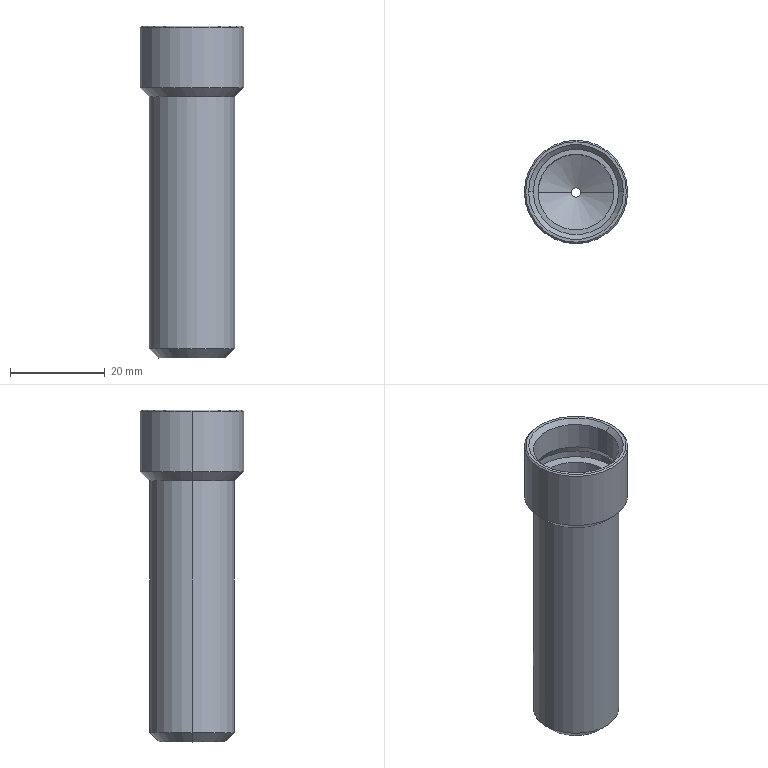Part | SolidWorks | features BaseBody 1 | 1 solid | 27 faces | box 21.8 x 21.8 x 70 mm | volume 5495 mm3 | cylinder 12 | cone 12 | plane 3 | commonest cylinder face diameters 18 x4 2 x2 16 x2 20 x2 21.8 x2
STEP:
#1=CARTESIAN_POINT('',(471.537,37.715,-74.634));
#2=VERTEX_POINT('',#1);
#3=CARTESIAN_POINT('',(489.537,37.715,-74.634));
#4=VERTEX_POINT('',#3);
#5=CARTESIAN_POINT('',(480.537,37.715,-74.634));
#6=DIRECTION('',(0.000000013,0.,-1.));
#7=DIRECTION('',(0.,1.,0.));
#8=AXIS2_PLACEMENT_3D('',#5,#6,#7);
#9=CIRCLE('',#8,9.);
#10=EDGE_CURVE('',#2,#4,#9,.T.);
#11=ORIENTED_EDGE('',*,*,#10,.F.);
#12=CARTESIAN_POINT('',(471.537,37.715,-21.534));
#13=VERTEX_POINT('',#12);
#14=CARTESIAN_POINT('',(471.537,37.715,-74.634));
#15=DIRECTION('',(-0.000000013,0.,1.));
#16=VECTOR('',#15,1000.);
#17=LINE('',#14,#16);
#18=EDGE_CURVE('',#2,#13,#17,.T.);
#19=ORIENTED_EDGE('',*,*,#18,.T.);
#20=CARTESIAN_POINT('',(489.537,37.715,-21.534));
#21=VERTEX_POINT('',#20);
#22=CARTESIAN_POINT('',(480.537,37.715,-21.534));
#23=DIRECTION('',(-0.000000013,0.,1.));
#24=DIRECTION('',(0.,1.,0.));
#25=AXIS2_PLACEMENT_3D('',#22,#23,#24);
#26=CIRCLE('',#25,9.);
#27=EDGE_CURVE('',#21,#13,#26,.T.);
#28=ORIENTED_EDGE('',*,*,#27,.F.);
#29=CARTESIAN_POINT('',(489.537,37.715,-74.634));
#30=DIRECTION('',(-0.000000013,0.,1.));
#31=VECTOR('',#30,1000.);
#32=LINE('',#29,#31);
#33=EDGE_CURVE('',#4,#21,#32,.T.);
#34=ORIENTED_EDGE('',*,*,#33,.F.);
#35=EDGE_LOOP('',(#11,#19,#28,#34));
#36=FACE_OUTER_BOUND('',#35,.T.);
#37=CARTESIAN_POINT('',(480.537,37.715,-74.634));
#38=DIRECTION('',(-0.000000013,0.,1.));
#39=DIRECTION('',(1.,0.,0.000000013));
#40=AXIS2_PLACEMENT_3D('',#37,#38,#39);
#41=CYLINDRICAL_SURFACE('',#40,9.);
#42=ADVANCED_FACE('',(#36),#41,.T.);
#43=CARTESIAN_POINT('',(473.537,37.715,-76.634));
#44=VERTEX_POINT('',#43);
#45=CARTESIAN_POINT('',(487.537,37.715,-76.634));
#46=VERTEX_POINT('',#45);
#47=CARTESIAN_POINT('',(480.537,37.715,-76.634));
#48=DIRECTION('',(0.000000013,0.,-1.));
#49=DIRECTION('',(1.,0.,0.000000013));
#50=AXIS2_PLACEMENT_3D('',#47,#48,#49);
#51=CIRCLE('',#50,7.);
#52=EDGE_CURVE('',#44,#46,#51,.T.);
#53=ORIENTED_EDGE('',*,*,#52,.F.);
#54=CARTESIAN_POINT('',(473.537,37.715,-76.634));
#55=DIRECTION('',(-0.7071,0.,0.7071));
#56=VECTOR('',#55,1000.);
#57=LINE('',#54,#56);
#58=EDGE_CURVE('',#44,#2,#57,.T.);
#59=ORIENTED_EDGE('',*,*,#58,.T.);
#60=ORIENTED_EDGE('',*,*,#10,.T.);
#61=CARTESIAN_POINT('',(487.537,37.715,-76.634));
#62=DIRECTION('',(0.7071,0.,0.7071));
#63=VECTOR('',#62,1000.);
#64=LINE('',#61,#63);
#65=EDGE_CURVE('',#46,#4,#64,.T.);
#66=ORIENTED_EDGE('',*,*,#65,.F.);
#67=EDGE_LOOP('',(#53,#59,#60,#66));
#68=FACE_OUTER_BOUND('',#67,.T.);
#69=CARTESIAN_POINT('',(480.537,37.715,-76.634));
#70=DIRECTION('',(-0.000000013,0.,1.));
#71=DIRECTION('',(1.,0.,0.000000013));
#72=AXIS2_PLACEMENT_3D('',#69,#70,#71);
#73=CONICAL_SURFACE('',#72,7.,0.7854);
#74=ADVANCED_FACE('',(#68),#73,.T.);
#75=ORIENTED_EDGE('',*,*,#27,.T.);
#76=CARTESIAN_POINT('',(469.637,37.715,-19.634));
#77=VERTEX_POINT('',#76);
#78=CARTESIAN_POINT('',(471.537,37.715,-21.534));
#79=DIRECTION('',(-0.7071,0.,0.7071));
#80=VECTOR('',#79,1000.);
#81=LINE('',#78,#80);
#82=EDGE_CURVE('',#13,#77,#81,.T.);
#83=ORIENTED_EDGE('',*,*,#82,.T.);
#84=CARTESIAN_POINT('',(491.437,37.715,-19.634));
#85=VERTEX_POINT('',#84);
#86=CARTESIAN_POINT('',(480.537,37.715,-19.634));
#87=DIRECTION('',(-0.000000013,0.,1.));
#88=DIRECTION('',(0.,1.,0.));
#89=AXIS2_PLACEMENT_3D('',#86,#87,#88);
#90=CIRCLE('',#89,10.9);
#91=EDGE_CURVE('',#85,#77,#90,.T.);
#92=ORIENTED_EDGE('',*,*,#91,.F.);
#93=CARTESIAN_POINT('',(489.537,37.715,-21.534));
#94=DIRECTION('',(0.7071,0.,0.7071));
#95=VECTOR('',#94,1000.);
#96=LINE('',#93,#95);
#97=EDGE_CURVE('',#21,#85,#96,.T.);
#98=ORIENTED_EDGE('',*,*,#97,.F.);
#99=EDGE_LOOP('',(#75,#83,#92,#98));
#100=FACE_OUTER_BOUND('',#99,.T.);
#101=CARTESIAN_POINT('',(480.537,37.715,-21.534));
#102=DIRECTION('',(-0.000000013,0.,1.));
#103=DIRECTION('',(1.,0.,0.000000013));
#104=AXIS2_PLACEMENT_3D('',#101,#102,#103);
#105=CONICAL_SURFACE('',#104,9.,0.7854);
#106=ADVANCED_FACE('',(#100),#105,.T.);
#107=ORIENTED_EDGE('',*,*,#91,.T.);
#108=CARTESIAN_POINT('',(469.637,37.715,-6.934));
#109=VERTEX_POINT('',#108);
#110=CARTESIAN_POINT('',(469.637,37.715,-19.634));
#111=DIRECTION('',(-0.000000013,0.,1.));
#112=VECTOR('',#111,1000.);
#113=LINE('',#110,#112);
#114=EDGE_CURVE('',#77,#109,#113,.T.);
#115=ORIENTED_EDGE('',*,*,#114,.T.);
#116=CARTESIAN_POINT('',(491.437,37.715,-6.934));
#117=VERTEX_POINT('',#116);
#118=CARTESIAN_POINT('',(480.537,37.715,-6.934));
#119=DIRECTION('',(-0.000000013,0.,1.));
#120=DIRECTION('',(0.,1.,0.));
#121=AXIS2_PLACEMENT_3D('',#118,#119,#120);
#122=CIRCLE('',#121,10.9);
#123=EDGE_CURVE('',#117,#109,#122,.T.);
#124=ORIENTED_EDGE('',*,*,#123,.F.);
#125=CARTESIAN_POINT('',(491.437,37.715,-19.634));
#126=DIRECTION('',(-0.000000013,0.,1.));
#127=VECTOR('',#126,1000.);
#128=LINE('',#125,#127);
#129=EDGE_CURVE('',#85,#117,#128,.T.);
#130=ORIENTED_EDGE('',*,*,#129,.F.);
#131=EDGE_LOOP('',(#107,#115,#124,#130));
#132=FACE_OUTER_BOUND('',#131,.T.);
#133=CARTESIAN_POINT('',(480.537,37.715,-19.634));
#134=DIRECTION('',(-0.000000013,0.,1.));
#135=DIRECTION('',(1.,0.,0.000000013));
#136=AXIS2_PLACEMENT_3D('',#133,#134,#135);
#137=CYLINDRICAL_SURFACE('',#136,10.9);
#138=ADVANCED_FACE('',(#132),#137,.T.);
#139=CARTESIAN_POINT('',(481.537,37.715,-76.634));
#140=VERTEX_POINT('',#139);
#141=CARTESIAN_POINT('',(479.537,37.715,-76.634));
#142=VERTEX_POINT('',#141);
#143=CARTESIAN_POINT('',(480.537,37.715,-76.634));
#144=DIRECTION('',(0.000000013,0.,-1.));
#145=DIRECTION('',(1.,0.,0.000000013));
#146=AXIS2_PLACEMENT_3D('',#143,#144,#145);
#147=CIRCLE('',#146,1.);
#148=EDGE_CURVE('',#140,#142,#147,.T.);
#149=ORIENTED_EDGE('',*,*,#148,.T.);
#150=CARTESIAN_POINT('',(479.537,37.715,-74.356));
#151=VERTEX_POINT('',#150);
#152=CARTESIAN_POINT('',(479.537,37.715,-76.634));
#153=DIRECTION('',(-0.000000013,0.,1.));
#154=VECTOR('',#153,1000.);
#155=LINE('',#152,#154);
#156=EDGE_CURVE('',#142,#151,#155,.T.);
#157=ORIENTED_EDGE('',*,*,#156,.T.);
#158=CARTESIAN_POINT('',(481.537,37.715,-74.356));
#159=VERTEX_POINT('',#158);
#160=CARTESIAN_POINT('',(480.537,37.715,-74.356));
#161=DIRECTION('',(-0.000000013,0.,1.));
#162=DIRECTION('',(0.,1.,0.));
#163=AXIS2_PLACEMENT_3D('',#160,#161,#162);
#164=CIRCLE('',#163,1.);
#165=EDGE_CURVE('',#151,#159,#164,.T.);
#166=ORIENTED_EDGE('',*,*,#165,.T.);
#167=CARTESIAN_POINT('',(481.537,37.715,-76.634));
#168=DIRECTION('',(-0.000000013,0.,1.));
#169=VECTOR('',#168,1000.);
#170=LINE('',#167,#169);
#171=EDGE_CURVE('',#140,#159,#170,.T.);
#172=ORIENTED_EDGE('',*,*,#171,.F.);
#173=EDGE_LOOP('',(#149,#157,#166,#172));
#174=FACE_OUTER_BOUND('',#173,.T.);
#175=CARTESIAN_POINT('',(480.537,37.715,-76.634));
#176=DIRECTION('',(-0.000000013,0.,1.));
#177=DIRECTION('',(1.,0.,0.000000013));
#178=AXIS2_PLACEMENT_3D('',#175,#176,#177);
#179=CYLINDRICAL_SURFACE('',#178,1.);
#180=ADVANCED_FACE('',(#174),#179,.F.);
#181=CARTESIAN_POINT('',(491.137,37.715,-6.634));
#182=VERTEX_POINT('',#181);
#183=CARTESIAN_POINT('',(469.937,37.715,-6.634));
#184=VERTEX_POINT('',#183);
#185=CARTESIAN_POINT('',(480.537,37.715,-6.634));
#186=DIRECTION('',(-0.000000013,0.,1.));
#187=DIRECTION('',(-1.,0.,-0.000000013));
#188=AXIS2_PLACEMENT_3D('',#185,#186,#187);
#189=CIRCLE('',#188,10.6);
#190=EDGE_CURVE('',#182,#184,#189,.T.);
#191=ORIENTED_EDGE('',*,*,#190,.F.);
#192=CARTESIAN_POINT('',(491.437,37.715,-6.934));
#193=DIRECTION('',(0.7071,0.,-0.7071));
#194=VECTOR('',#193,1000.);
#195=LINE('',#192,#194);
#196=EDGE_CURVE('',#182,#117,#195,.T.);
#197=ORIENTED_EDGE('',*,*,#196,.T.);
#198=ORIENTED_EDGE('',*,*,#123,.T.);
#199=CARTESIAN_POINT('',(469.637,37.715,-6.934));
#200=DIRECTION('',(-0.7071,0.,-0.7071));
#201=VECTOR('',#200,1000.);
#202=LINE('',#199,#201);
#203=EDGE_CURVE('',#184,#109,#202,.T.);
#204=ORIENTED_EDGE('',*,*,#203,.F.);
#205=EDGE_LOOP('',(#191,#197,#198,#204));
#206=FACE_OUTER_BOUND('',#205,.T.);
#207=CARTESIAN_POINT('',(480.537,37.715,-6.934));
#208=DIRECTION('',(0.000000013,0.,-1.));
#209=DIRECTION('',(-1.,0.,-0.000000013));
#210=AXIS2_PLACEMENT_3D('',#207,#208,#209);
#211=CONICAL_SURFACE('',#210,10.9,0.7854);
#212=ADVANCED_FACE('',(#206),#211,.T.);
#213=ORIENTED_EDGE('',*,*,#165,.F.);
#214=CARTESIAN_POINT('',(472.537,37.715,-70.634));
#215=VERTEX_POINT('',#214);
#216=CARTESIAN_POINT('',(479.537,37.715,-74.356));
#217=DIRECTION('',(-0.8829,0.,0.4695));
#218=VECTOR('',#217,1000.);
#219=LINE('',#216,#218);
#220=EDGE_CURVE('',#151,#215,#219,.T.);
#221=ORIENTED_EDGE('',*,*,#220,.T.);
#222=CARTESIAN_POINT('',(488.537,37.715,-70.634));
#223=VERTEX_POINT('',#222);
#224=CARTESIAN_POINT('',(480.537,37.715,-70.634));
#225=DIRECTION('',(-0.000000013,0.,1.));
#226=DIRECTION('',(0.,1.,0.));
#227=AXIS2_PLACEMENT_3D('',#224,#225,#226);
#228=CIRCLE('',#227,8.);
#229=EDGE_CURVE('',#215,#223,#228,.T.);
#230=ORIENTED_EDGE('',*,*,#229,.T.);
#231=CARTESIAN_POINT('',(481.537,37.715,-74.356));
#232=DIRECTION('',(0.8829,0.,0.4695));
#233=VECTOR('',#232,1000.);
#234=LINE('',#231,#233);
#235=EDGE_CURVE('',#159,#223,#234,.T.);
#236=ORIENTED_EDGE('',*,*,#235,.F.);
#237=EDGE_LOOP('',(#213,#221,#230,#236));
#238=FACE_OUTER_BOUND('',#237,.T.);
#239=CARTESIAN_POINT('',(480.537,37.715,-74.356));
#240=DIRECTION('',(-0.000000013,0.,1.));
#241=DIRECTION('',(1.,0.,0.000000013));
#242=AXIS2_PLACEMENT_3D('',#239,#240,#241);
#243=CONICAL_SURFACE('',#242,1.,1.082);
#244=ADVANCED_FACE('',(#238),#243,.F.);
#245=ORIENTED_EDGE('',*,*,#229,.F.);
#246=CARTESIAN_POINT('',(472.537,37.715,-16.634));
#247=VERTEX_POINT('',#246);
#248=CARTESIAN_POINT('',(472.537,37.715,-70.634));
#249=DIRECTION('',(-0.000000013,0.,1.));
#250=VECTOR('',#249,1000.);
#251=LINE('',#248,#250);
#252=EDGE_CURVE('',#215,#247,#251,.T.);
#253=ORIENTED_EDGE('',*,*,#252,.T.);
#254=CARTESIAN_POINT('',(488.537,37.715,-16.634));
#255=VERTEX_POINT('',#254);
#256=CARTESIAN_POINT('',(480.537,37.715,-16.634));
#257=DIRECTION('',(-0.000000013,0.,1.));
#258=DIRECTION('',(1.,0.,0.000000013));
#259=AXIS2_PLACEMENT_3D('',#256,#257,#258);
#260=CIRCLE('',#259,8.);
#261=EDGE_CURVE('',#247,#255,#260,.T.);
#262=ORIENTED_EDGE('',*,*,#261,.T.);
#263=CARTESIAN_POINT('',(488.537,37.715,-70.634));
#264=DIRECTION('',(-0.000000013,0.,1.));
#265=VECTOR('',#264,1000.);
#266=LINE('',#263,#265);
#267=EDGE_CURVE('',#223,#255,#266,.T.);
#268=ORIENTED_EDGE('',*,*,#267,.F.);
#269=EDGE_LOOP('',(#245,#253,#262,#268));
#270=FACE_OUTER_BOUND('',#269,.T.);
#271=CARTESIAN_POINT('',(480.537,37.715,-70.634));
#272=DIRECTION('',(-0.000000013,0.,1.));
#273=DIRECTION('',(1.,0.,0.000000013));
#274=AXIS2_PLACEMENT_3D('',#271,#272,#273);
#275=CYLINDRICAL_SURFACE('',#274,8.);
#276=ADVANCED_FACE('',(#270),#275,.F.);
#277=CARTESIAN_POINT('',(489.537,37.715,-7.634));
#278=VERTEX_POINT('',#277);
#279=CARTESIAN_POINT('',(471.537,37.715,-7.634));
#280=VERTEX_POINT('',#279);
#281=CARTESIAN_POINT('',(480.537,37.715,-7.634));
#282=DIRECTION('',(0.000000013,0.,-1.));
#283=DIRECTION('',(0.,1.,0.));
#284=AXIS2_PLACEMENT_3D('',#281,#282,#283);
#285=CIRCLE('',#284,9.);
#286=EDGE_CURVE('',#278,#280,#285,.T.);
#287=ORIENTED_EDGE('',*,*,#286,.T.);
#288=CARTESIAN_POINT('',(470.537,37.715,-6.634));
#289=VERTEX_POINT('',#288);
#290=CARTESIAN_POINT('',(471.537,37.715,-7.634));
#291=DIRECTION('',(-0.7071,0.,0.7071));
#292=VECTOR('',#291,1000.);
#293=LINE('',#290,#292);
#294=EDGE_CURVE('',#280,#289,#293,.T.);
#295=ORIENTED_EDGE('',*,*,#294,.T.);
#296=CARTESIAN_POINT('',(490.537,37.715,-6.634));
#297=VERTEX_POINT('',#296);
#298=CARTESIAN_POINT('',(480.537,37.715,-6.634));
#299=DIRECTION('',(0.000000013,0.,-1.));
#300=DIRECTION('',(1.,0.,0.000000013));
#301=AXIS2_PLACEMENT_3D('',#298,#299,#300);
#302=CIRCLE('',#301,10.);
#303=EDGE_CURVE('',#297,#289,#302,.T.);
#304=ORIENTED_EDGE('',*,*,#303,.F.);
#305=CARTESIAN_POINT('',(489.537,37.715,-7.634));
#306=DIRECTION('',(0.7071,0.,0.7071));
#307=VECTOR('',#306,1000.);
#308=LINE('',#305,#307);
#309=EDGE_CURVE('',#278,#297,#308,.T.);
#310=ORIENTED_EDGE('',*,*,#309,.F.);
#311=EDGE_LOOP('',(#287,#295,#304,#310));
#312=FACE_OUTER_BOUND('',#311,.T.);
#313=CARTESIAN_POINT('',(480.537,37.715,-7.634));
#314=DIRECTION('',(-0.000000013,0.,1.));
#315=DIRECTION('',(1.,0.,0.000000013));
#316=AXIS2_PLACEMENT_3D('',#313,#314,#315);
#317=CONICAL_SURFACE('',#316,9.,0.7854);
#318=ADVANCED_FACE('',(#312),#317,.F.);
#319=CARTESIAN_POINT('',(489.537,37.715,-13.402));
#320=VERTEX_POINT('',#319);
#321=CARTESIAN_POINT('',(471.537,37.715,-13.402));
#322=VERTEX_POINT('',#321);
#323=CARTESIAN_POINT('',(480.537,37.715,-13.402));
#324=DIRECTION('',(0.000000013,0.,-1.));
#325=DIRECTION('',(0.,1.,0.));
#326=AXIS2_PLACEMENT_3D('',#323,#324,#325);
#327=CIRCLE('',#326,9.);
#328=EDGE_CURVE('',#320,#322,#327,.T.);
#329=ORIENTED_EDGE('',*,*,#328,.T.);
#330=CARTESIAN_POINT('',(471.537,37.715,-13.402));
#331=DIRECTION('',(-0.000000013,0.,1.));
#332=VECTOR('',#331,1000.);
#333=LINE('',#330,#332);
#334=EDGE_CURVE('',#322,#280,#333,.T.);
#335=ORIENTED_EDGE('',*,*,#334,.T.);
#336=ORIENTED_EDGE('',*,*,#286,.F.);
#337=CARTESIAN_POINT('',(489.537,37.715,-13.402));
#338=DIRECTION('',(-0.000000013,0.,1.));
#339=VECTOR('',#338,1000.);
#340=LINE('',#337,#339);
#341=EDGE_CURVE('',#320,#278,#340,.T.);
#342=ORIENTED_EDGE('',*,*,#341,.F.);
#343=EDGE_LOOP('',(#329,#335,#336,#342));
#344=FACE_OUTER_BOUND('',#343,.T.);
#345=CARTESIAN_POINT('',(480.537,37.715,-13.402));
#346=DIRECTION('',(-0.000000013,0.,1.));
#347=DIRECTION('',(1.,0.,0.000000013));
#348=AXIS2_PLACEMENT_3D('',#345,#346,#347);
#349=CYLINDRICAL_SURFACE('',#348,9.);
#350=ADVANCED_FACE('',(#344),#349,.F.);
#351=CARTESIAN_POINT('',(470.537,37.715,-16.634));
#352=VERTEX_POINT('',#351);
#353=CARTESIAN_POINT('',(490.537,37.715,-16.634));
#354=VERTEX_POINT('',#353);
#355=CARTESIAN_POINT('',(480.537,37.715,-16.634));
#356=DIRECTION('',(-0.000000013,0.,1.));
#357=DIRECTION('',(1.,0.,0.000000013));
#358=AXIS2_PLACEMENT_3D('',#355,#356,#357);
#359=CIRCLE('',#358,10.);
#360=EDGE_CURVE('',#352,#354,#359,.T.);
#361=ORIENTED_EDGE('',*,*,#360,.F.);
#362=CARTESIAN_POINT('',(470.537,37.715,-15.134));
#363=VERTEX_POINT('',#362);
#364=CARTESIAN_POINT('',(470.537,37.715,-16.634));
#365=DIRECTION('',(-0.000000013,0.,1.));
#366=VECTOR('',#365,1000.);
#367=LINE('',#364,#366);
#368=EDGE_CURVE('',#352,#363,#367,.T.);
#369=ORIENTED_EDGE('',*,*,#368,.T.);
#370=CARTESIAN_POINT('',(490.537,37.715,-15.134));
#371=VERTEX_POINT('',#370);
#372=CARTESIAN_POINT('',(480.537,37.715,-15.134));
#373=DIRECTION('',(-0.000000013,0.,1.));
#374=DIRECTION('',(0.,1.,0.));
#375=AXIS2_PLACEMENT_3D('',#372,#373,#374);
#376=CIRCLE('',#375,10.);
#377=EDGE_CURVE('',#363,#371,#376,.T.);
#378=ORIENTED_EDGE('',*,*,#377,.T.);
#379=CARTESIAN_POINT('',(490.537,37.715,-16.634));
#380=DIRECTION('',(-0.000000013,0.,1.));
#381=VECTOR('',#380,1000.);
#382=LINE('',#379,#381);
#383=EDGE_CURVE('',#354,#371,#382,.T.);
#384=ORIENTED_EDGE('',*,*,#383,.F.);
#385=EDGE_LOOP('',(#361,#369,#378,#384));
#386=FACE_OUTER_BOUND('',#385,.T.);
#387=CARTESIAN_POINT('',(480.537,37.715,-16.634));
#388=DIRECTION('',(-0.000000013,0.,1.));
#389=DIRECTION('',(1.,0.,0.000000013));
#390=AXIS2_PLACEMENT_3D('',#387,#388,#389);
#391=CYLINDRICAL_SURFACE('',#390,10.);
#392=ADVANCED_FACE('',(#386),#391,.F.);
#393=ORIENTED_EDGE('',*,*,#328,.F.);
#394=CARTESIAN_POINT('',(490.537,37.715,-15.134));
#395=DIRECTION('',(0.5,0.,-0.866));
#396=VECTOR('',#395,1000.);
#397=LINE('',#394,#396);
#398=EDGE_CURVE('',#320,#371,#397,.T.);
#399=ORIENTED_EDGE('',*,*,#398,.T.);
#400=ORIENTED_EDGE('',*,*,#377,.F.);
#401=CARTESIAN_POINT('',(470.537,37.715,-15.134));
#402=DIRECTION('',(-0.5,0.,-0.866));
#403=VECTOR('',#402,1000.);
#404=LINE('',#401,#403);
#405=EDGE_CURVE('',#322,#363,#404,.T.);
#406=ORIENTED_EDGE('',*,*,#405,.F.);
#407=EDGE_LOOP('',(#393,#399,#400,#406));
#408=FACE_OUTER_BOUND('',#407,.T.);
#409=CARTESIAN_POINT('',(480.537,37.715,-15.134));
#410=DIRECTION('',(0.000000013,0.,-1.));
#411=DIRECTION('',(-1.,0.,-0.000000013));
#412=AXIS2_PLACEMENT_3D('',#409,#410,#411);
#413=CONICAL_SURFACE('',#412,10.,0.5236);
#414=ADVANCED_FACE('',(#408),#413,.F.);
#415=ORIENTED_EDGE('',*,*,#18,.F.);
#416=CARTESIAN_POINT('',(480.537,37.715,-74.634));
#417=DIRECTION('',(0.000000013,0.,-1.));
#418=DIRECTION('',(0.,1.,0.));
#419=AXIS2_PLACEMENT_3D('',#416,#417,#418);
#420=CIRCLE('',#419,9.);
#421=EDGE_CURVE('',#4,#2,#420,.T.);
#422=ORIENTED_EDGE('',*,*,#421,.F.);
#423=ORIENTED_EDGE('',*,*,#33,.T.);
#424=CARTESIAN_POINT('',(480.537,37.715,-21.534));
#425=DIRECTION('',(-0.000000013,0.,1.));
#426=DIRECTION('',(0.,1.,0.));
#427=AXIS2_PLACEMENT_3D('',#424,#425,#426);
#428=CIRCLE('',#427,9.);
#429=EDGE_CURVE('',#13,#21,#428,.T.);
#430=ORIENTED_EDGE('',*,*,#429,.F.);
#431=EDGE_LOOP('',(#415,#422,#423,#430));
#432=FACE_OUTER_BOUND('',#431,.T.);
#433=CARTESIAN_POINT('',(480.537,37.715,-74.634));
#434=DIRECTION('',(-0.000000013,0.,1.));
#435=DIRECTION('',(1.,0.,0.000000013));
#436=AXIS2_PLACEMENT_3D('',#433,#434,#435);
#437=CYLINDRICAL_SURFACE('',#436,9.);
#438=ADVANCED_FACE('',(#432),#437,.T.);
#439=ORIENTED_EDGE('',*,*,#58,.F.);
#440=CARTESIAN_POINT('',(480.537,37.715,-76.634));
#441=DIRECTION('',(0.000000013,0.,-1.));
#442=DIRECTION('',(1.,0.,0.000000013));
#443=AXIS2_PLACEMENT_3D('',#440,#441,#442);
#444=CIRCLE('',#443,7.);
#445=EDGE_CURVE('',#46,#44,#444,.T.);
#446=ORIENTED_EDGE('',*,*,#445,.F.);
#447=ORIENTED_EDGE('',*,*,#65,.T.);
#448=ORIENTED_EDGE('',*,*,#421,.T.);
#449=EDGE_LOOP('',(#439,#446,#447,#448));
#450=FACE_OUTER_BOUND('',#449,.T.);
#451=CARTESIAN_POINT('',(480.537,37.715,-76.634));
#452=DIRECTION('',(-0.000000013,0.,1.));
#453=DIRECTION('',(1.,0.,0.000000013));
#454=AXIS2_PLACEMENT_3D('',#451,#452,#453);
#455=CONICAL_SURFACE('',#454,7.,0.7854);
#456=ADVANCED_FACE('',(#450),#455,.T.);
#457=ORIENTED_EDGE('',*,*,#82,.F.);
#458=ORIENTED_EDGE('',*,*,#429,.T.);
#459=ORIENTED_EDGE('',*,*,#97,.T.);
#460=CARTESIAN_POINT('',(480.537,37.715,-19.634));
#461=DIRECTION('',(-0.000000013,0.,1.));
#462=DIRECTION('',(0.,1.,0.));
#463=AXIS2_PLACEMENT_3D('',#460,#461,#462);
#464=CIRCLE('',#463,10.9);
#465=EDGE_CURVE('',#77,#85,#464,.T.);
#466=ORIENTED_EDGE('',*,*,#465,.F.);
#467=EDGE_LOOP('',(#457,#458,#459,#466));
#468=FACE_OUTER_BOUND('',#467,.T.);
#469=CARTESIAN_POINT('',(480.537,37.715,-21.534));
#470=DIRECTION('',(-0.000000013,0.,1.));
#471=DIRECTION('',(1.,0.,0.000000013));
#472=AXIS2_PLACEMENT_3D('',#469,#470,#471);
#473=CONICAL_SURFACE('',#472,9.,0.7854);
#474=ADVANCED_FACE('',(#468),#473,.T.);
#475=ORIENTED_EDGE('',*,*,#148,.F.);
#476=CARTESIAN_POINT('',(480.537,37.715,-76.634));
#477=DIRECTION('',(0.000000013,0.,-1.));
#478=DIRECTION('',(1.,0.,0.000000013));
#479=AXIS2_PLACEMENT_3D('',#476,#477,#478);
#480=CIRCLE('',#479,1.);
#481=EDGE_CURVE('',#142,#140,#480,.T.);
#482=ORIENTED_EDGE('',*,*,#481,.F.);
#483=EDGE_LOOP('',(#475,#482));
#484=FACE_BOUND('',#483,.T.);
#485=ORIENTED_EDGE('',*,*,#445,.T.);
#486=ORIENTED_EDGE('',*,*,#52,.T.);
#487=EDGE_LOOP('',(#485,#486));
#488=FACE_OUTER_BOUND('',#487,.T.);
#489=CARTESIAN_POINT('',(487.817,30.435,-76.634));
#490=DIRECTION('',(-0.000000013,0.,1.));
#491=DIRECTION('',(0.,1.,0.));
#492=AXIS2_PLACEMENT_3D('',#489,#490,#491);
#493=PLANE('',#492);
#494=ADVANCED_FACE('',(#484,#488),#493,.F.);
#495=ORIENTED_EDGE('',*,*,#114,.F.);
#496=ORIENTED_EDGE('',*,*,#465,.T.);
#497=ORIENTED_EDGE('',*,*,#129,.T.);
#498=CARTESIAN_POINT('',(480.537,37.715,-6.934));
#499=DIRECTION('',(-0.000000013,0.,1.));
#500=DIRECTION('',(0.,1.,0.));
#501=AXIS2_PLACEMENT_3D('',#498,#499,#500);
#502=CIRCLE('',#501,10.9);
#503=EDGE_CURVE('',#109,#117,#502,.T.);
#504=ORIENTED_EDGE('',*,*,#503,.F.);
#505=EDGE_LOOP('',(#495,#496,#497,#504));
#506=FACE_OUTER_BOUND('',#505,.T.);
#507=CARTESIAN_POINT('',(480.537,37.715,-19.634));
#508=DIRECTION('',(-0.000000013,0.,1.));
#509=DIRECTION('',(1.,0.,0.000000013));
#510=AXIS2_PLACEMENT_3D('',#507,#508,#509);
#511=CYLINDRICAL_SURFACE('',#510,10.9);
#512=ADVANCED_FACE('',(#506),#511,.T.);
#513=ORIENTED_EDGE('',*,*,#156,.F.);
#514=ORIENTED_EDGE('',*,*,#481,.T.);
#515=ORIENTED_EDGE('',*,*,#171,.T.);
#516=CARTESIAN_POINT('',(480.537,37.715,-74.356));
#517=DIRECTION('',(-0.000000013,0.,1.));
#518=DIRECTION('',(0.,1.,0.));
#519=AXIS2_PLACEMENT_3D('',#516,#517,#518);
#520=CIRCLE('',#519,1.);
#521=EDGE_CURVE('',#159,#151,#520,.T.);
#522=ORIENTED_EDGE('',*,*,#521,.T.);
#523=EDGE_LOOP('',(#513,#514,#515,#522));
#524=FACE_OUTER_BOUND('',#523,.T.);
#525=CARTESIAN_POINT('',(480.537,37.715,-76.634));
#526=DIRECTION('',(-0.000000013,0.,1.));
#527=DIRECTION('',(1.,0.,0.000000013));
#528=AXIS2_PLACEMENT_3D('',#525,#526,#527);
#529=CYLINDRICAL_SURFACE('',#528,1.);
#530=ADVANCED_FACE('',(#524),#529,.F.);
#531=ORIENTED_EDGE('',*,*,#196,.F.);
#532=CARTESIAN_POINT('',(480.537,37.715,-6.634));
#533=DIRECTION('',(-0.000000013,0.,1.));
#534=DIRECTION('',(-1.,0.,-0.000000013));
#535=AXIS2_PLACEMENT_3D('',#532,#533,#534);
#536=CIRCLE('',#535,10.6);
#537=EDGE_CURVE('',#184,#182,#536,.T.);
#538=ORIENTED_EDGE('',*,*,#537,.F.);
#539=ORIENTED_EDGE('',*,*,#203,.T.);
#540=ORIENTED_EDGE('',*,*,#503,.T.);
#541=EDGE_LOOP('',(#531,#538,#539,#540));
#542=FACE_OUTER_BOUND('',#541,.T.);
#543=CARTESIAN_POINT('',(480.537,37.715,-6.934));
#544=DIRECTION('',(0.000000013,0.,-1.));
#545=DIRECTION('',(-1.,0.,-0.000000013));
#546=AXIS2_PLACEMENT_3D('',#543,#544,#545);
#547=CONICAL_SURFACE('',#546,10.9,0.7854);
#548=ADVANCED_FACE('',(#542),#547,.T.);
#549=ORIENTED_EDGE('',*,*,#220,.F.);
#550=ORIENTED_EDGE('',*,*,#521,.F.);
#551=ORIENTED_EDGE('',*,*,#235,.T.);
#552=CARTESIAN_POINT('',(480.537,37.715,-70.634));
#553=DIRECTION('',(-0.000000013,0.,1.));
#554=DIRECTION('',(0.,1.,0.));
#555=AXIS2_PLACEMENT_3D('',#552,#553,#554);
#556=CIRCLE('',#555,8.);
#557=EDGE_CURVE('',#223,#215,#556,.T.);
#558=ORIENTED_EDGE('',*,*,#557,.T.);
#559=EDGE_LOOP('',(#549,#550,#551,#558));
#560=FACE_OUTER_BOUND('',#559,.T.);
#561=CARTESIAN_POINT('',(480.537,37.715,-74.356));
#562=DIRECTION('',(-0.000000013,0.,1.));
#563=DIRECTION('',(1.,0.,0.000000013));
#564=AXIS2_PLACEMENT_3D('',#561,#562,#563);
#565=CONICAL_SURFACE('',#564,1.,1.082);
#566=ADVANCED_FACE('',(#560),#565,.F.);
#567=ORIENTED_EDGE('',*,*,#303,.T.);
#568=CARTESIAN_POINT('',(480.537,37.715,-6.634));
#569=DIRECTION('',(0.000000013,0.,-1.));
#570=DIRECTION('',(1.,0.,0.000000013));
#571=AXIS2_PLACEMENT_3D('',#568,#569,#570);
#572=CIRCLE('',#571,10.);
#573=EDGE_CURVE('',#289,#297,#572,.T.);
#574=ORIENTED_EDGE('',*,*,#573,.T.);
#575=EDGE_LOOP('',(#567,#574));
#576=FACE_BOUND('',#575,.T.);
#577=ORIENTED_EDGE('',*,*,#537,.T.);
#578=ORIENTED_EDGE('',*,*,#190,.T.);
#579=EDGE_LOOP('',(#577,#578));
#580=FACE_OUTER_BOUND('',#579,.T.);
#581=CARTESIAN_POINT('',(491.575,26.691,-6.634));
#582=DIRECTION('',(-0.000000013,0.,1.));
#583=DIRECTION('',(0.,1.,0.));
#584=AXIS2_PLACEMENT_3D('',#581,#582,#583);
#585=PLANE('',#584);
#586=ADVANCED_FACE('',(#576,#580),#585,.T.);
#587=ORIENTED_EDGE('',*,*,#252,.F.);
#588=ORIENTED_EDGE('',*,*,#557,.F.);
#589=ORIENTED_EDGE('',*,*,#267,.T.);
#590=CARTESIAN_POINT('',(480.537,37.715,-16.634));
#591=DIRECTION('',(-0.000000013,0.,1.));
#592=DIRECTION('',(1.,0.,0.000000013));
#593=AXIS2_PLACEMENT_3D('',#590,#591,#592);
#594=CIRCLE('',#593,8.);
#595=EDGE_CURVE('',#255,#247,#594,.T.);
#596=ORIENTED_EDGE('',*,*,#595,.T.);
#597=EDGE_LOOP('',(#587,#588,#589,#596));
#598=FACE_OUTER_BOUND('',#597,.T.);
#599=CARTESIAN_POINT('',(480.537,37.715,-70.634));
#600=DIRECTION('',(-0.000000013,0.,1.));
#601=DIRECTION('',(1.,0.,0.000000013));
#602=AXIS2_PLACEMENT_3D('',#599,#600,#601);
#603=CYLINDRICAL_SURFACE('',#602,8.);
#604=ADVANCED_FACE('',(#598),#603,.F.);
#605=ORIENTED_EDGE('',*,*,#294,.F.);
#606=CARTESIAN_POINT('',(480.537,37.715,-7.634));
#607=DIRECTION('',(0.000000013,0.,-1.));
#608=DIRECTION('',(0.,1.,0.));
#609=AXIS2_PLACEMENT_3D('',#606,#607,#608);
#610=CIRCLE('',#609,9.);
#611=EDGE_CURVE('',#280,#278,#610,.T.);
#612=ORIENTED_EDGE('',*,*,#611,.T.);
#613=ORIENTED_EDGE('',*,*,#309,.T.);
#614=ORIENTED_EDGE('',*,*,#573,.F.);
#615=EDGE_LOOP('',(#605,#612,#613,#614));
#616=FACE_OUTER_BOUND('',#615,.T.);
#617=CARTESIAN_POINT('',(480.537,37.715,-7.634));
#618=DIRECTION('',(-0.000000013,0.,1.));
#619=DIRECTION('',(1.,0.,0.000000013));
#620=AXIS2_PLACEMENT_3D('',#617,#618,#619);
#621=CONICAL_SURFACE('',#620,9.,0.7854);
#622=ADVANCED_FACE('',(#616),#621,.F.);
#623=ORIENTED_EDGE('',*,*,#595,.F.);
#624=ORIENTED_EDGE('',*,*,#261,.F.);
#625=EDGE_LOOP('',(#623,#624));
#626=FACE_BOUND('',#625,.T.);
#627=CARTESIAN_POINT('',(480.537,37.715,-16.634));
#628=DIRECTION('',(-0.000000013,0.,1.));
#629=DIRECTION('',(1.,0.,0.000000013));
#630=AXIS2_PLACEMENT_3D('',#627,#628,#629);
#631=CIRCLE('',#630,10.);
#632=EDGE_CURVE('',#354,#352,#631,.T.);
#633=ORIENTED_EDGE('',*,*,#632,.T.);
#634=ORIENTED_EDGE('',*,*,#360,.T.);
#635=EDGE_LOOP('',(#633,#634));
#636=FACE_OUTER_BOUND('',#635,.T.);
#637=CARTESIAN_POINT('',(490.95,27.315,-16.634));
#638=DIRECTION('',(-0.000000013,0.,1.));
#639=DIRECTION('',(0.,1.,0.));
#640=AXIS2_PLACEMENT_3D('',#637,#638,#639);
#641=PLANE('',#640);
#642=ADVANCED_FACE('',(#626,#636),#641,.T.);
#643=ORIENTED_EDGE('',*,*,#334,.F.);
#644=CARTESIAN_POINT('',(480.537,37.715,-13.402));
#645=DIRECTION('',(0.000000013,0.,-1.));
#646=DIRECTION('',(0.,1.,0.));
#647=AXIS2_PLACEMENT_3D('',#644,#645,#646);
#648=CIRCLE('',#647,9.);
#649=EDGE_CURVE('',#322,#320,#648,.T.);
#650=ORIENTED_EDGE('',*,*,#649,.T.);
#651=ORIENTED_EDGE('',*,*,#341,.T.);
#652=ORIENTED_EDGE('',*,*,#611,.F.);
#653=EDGE_LOOP('',(#643,#650,#651,#652));
#654=FACE_OUTER_BOUND('',#653,.T.);
#655=CARTESIAN_POINT('',(480.537,37.715,-13.402));
#656=DIRECTION('',(-0.000000013,0.,1.));
#657=DIRECTION('',(1.,0.,0.000000013));
#658=AXIS2_PLACEMENT_3D('',#655,#656,#657);
#659=CYLINDRICAL_SURFACE('',#658,9.);
#660=ADVANCED_FACE('',(#654),#659,.F.);
#661=ORIENTED_EDGE('',*,*,#368,.F.);
#662=ORIENTED_EDGE('',*,*,#632,.F.);
#663=ORIENTED_EDGE('',*,*,#383,.T.);
#664=CARTESIAN_POINT('',(480.537,37.715,-15.134));
#665=DIRECTION('',(-0.000000013,0.,1.));
#666=DIRECTION('',(0.,1.,0.));
#667=AXIS2_PLACEMENT_3D('',#664,#665,#666);
#668=CIRCLE('',#667,10.);
#669=EDGE_CURVE('',#371,#363,#668,.T.);
#670=ORIENTED_EDGE('',*,*,#669,.T.);
#671=EDGE_LOOP('',(#661,#662,#663,#670));
#672=FACE_OUTER_BOUND('',#671,.T.);
#673=CARTESIAN_POINT('',(480.537,37.715,-16.634));
#674=DIRECTION('',(-0.000000013,0.,1.));
#675=DIRECTION('',(1.,0.,0.000000013));
#676=AXIS2_PLACEMENT_3D('',#673,#674,#675);
#677=CYLINDRICAL_SURFACE('',#676,10.);
#678=ADVANCED_FACE('',(#672),#677,.F.);
#679=ORIENTED_EDGE('',*,*,#398,.F.);
#680=ORIENTED_EDGE('',*,*,#649,.F.);
#681=ORIENTED_EDGE('',*,*,#405,.T.);
#682=ORIENTED_EDGE('',*,*,#669,.F.);
#683=EDGE_LOOP('',(#679,#680,#681,#682));
#684=FACE_OUTER_BOUND('',#683,.T.);
#685=CARTESIAN_POINT('',(480.537,37.715,-15.134));
#686=DIRECTION('',(0.000000013,0.,-1.));
#687=DIRECTION('',(-1.,0.,-0.000000013));
#688=AXIS2_PLACEMENT_3D('',#685,#686,#687);
#689=CONICAL_SURFACE('',#688,10.,0.5236);
#690=ADVANCED_FACE('',(#684),#689,.F.);
#691=CLOSED_SHELL('',(#42,#74,#106,#138,#180,#212,#244,#276,#318,#350,#392,#414,#438,#456,#474,#494,#512,#530,#548,#566,#586,#604,#622,#642,#660,#678,#690));
#692=MANIFOLD_SOLID_BREP('',#691);
#693=CARTESIAN_POINT('',(0.,0.,0.));
#694=DIRECTION('',(0.,0.,1.));
#695=DIRECTION('',(1.,0.,0.));
#696=AXIS2_PLACEMENT_3D('',#693,#694,#695);
#697=(LENGTH_UNIT()NAMED_UNIT(*)SI_UNIT(.MILLI.,.METRE.));
#698=UNCERTAINTY_MEASURE_WITH_UNIT(LENGTH_MEASURE(0.00001),#697,'','');
#699=(NAMED_UNIT(*)PLANE_ANGLE_UNIT()SI_UNIT($,.RADIAN.));
#700=(NAMED_UNIT(*)SI_UNIT($,.STERADIAN.)SOLID_ANGLE_UNIT());
#701=(GEOMETRIC_REPRESENTATION_CONTEXT(3)GLOBAL_UNCERTAINTY_ASSIGNED_CONTEXT((#698))GLOBAL_UNIT_ASSIGNED_CONTEXT((#697,#699,#700))REPRESENTATION_CONTEXT('',''));
#702=ADVANCED_BREP_SHAPE_REPRESENTATION('',(#692,#696),#701);